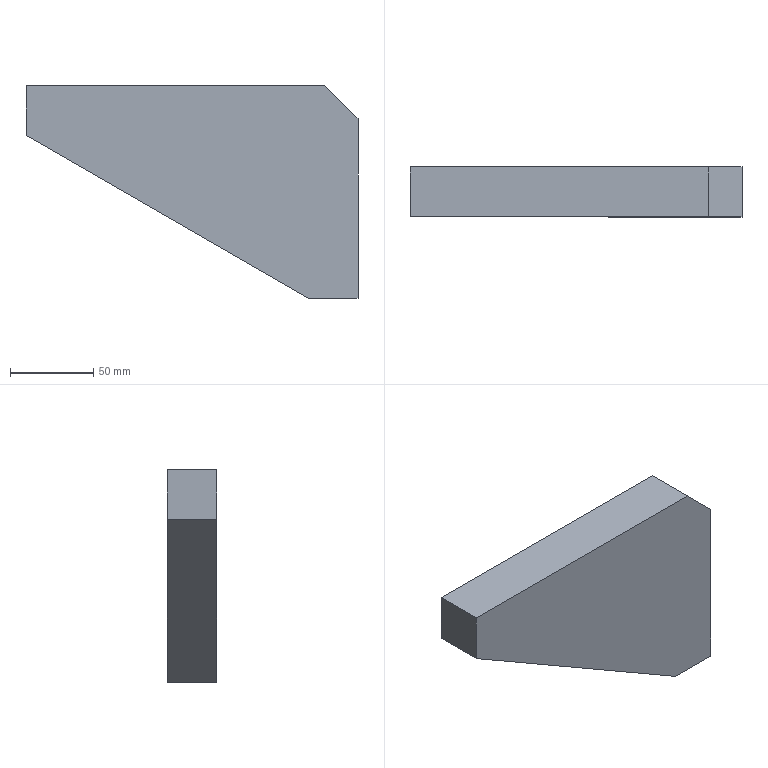Part | SolidWorks | features Extrusion 1 | 1 solid | 8 faces | box 200 x 30 x 128.15 mm | volume 512616 mm3 | plane 8
STEP:
#1=CARTESIAN_POINT('',(0.,0.,108.15));
#2=VERTEX_POINT('',#1);
#3=CARTESIAN_POINT('',(0.,0.,0.));
#4=VERTEX_POINT('',#3);
#5=CARTESIAN_POINT('',(0.,0.,108.15));
#6=DIRECTION('',(0.,0.,-1.));
#7=VECTOR('',#6,1000.);
#8=LINE('',#5,#7);
#9=EDGE_CURVE('',#2,#4,#8,.T.);
#10=ORIENTED_EDGE('',*,*,#9,.T.);
#11=CARTESIAN_POINT('',(0.,30.,0.));
#12=VERTEX_POINT('',#11);
#13=CARTESIAN_POINT('',(0.,30.,0.));
#14=DIRECTION('',(0.,-1.,0.));
#15=VECTOR('',#14,1000.);
#16=LINE('',#13,#15);
#17=EDGE_CURVE('',#12,#4,#16,.T.);
#18=ORIENTED_EDGE('',*,*,#17,.F.);
#19=CARTESIAN_POINT('',(0.,30.,108.15));
#20=VERTEX_POINT('',#19);
#21=CARTESIAN_POINT('',(0.,30.,108.15));
#22=DIRECTION('',(0.,0.,-1.));
#23=VECTOR('',#22,1000.);
#24=LINE('',#21,#23);
#25=EDGE_CURVE('',#20,#12,#24,.T.);
#26=ORIENTED_EDGE('',*,*,#25,.F.);
#27=CARTESIAN_POINT('',(0.,30.,108.15));
#28=DIRECTION('',(0.,-1.,0.));
#29=VECTOR('',#28,1000.);
#30=LINE('',#27,#29);
#31=EDGE_CURVE('',#20,#2,#30,.T.);
#32=ORIENTED_EDGE('',*,*,#31,.T.);
#33=EDGE_LOOP('',(#10,#18,#26,#32));
#34=FACE_OUTER_BOUND('',#33,.T.);
#35=CARTESIAN_POINT('',(0.,30.,108.15));
#36=DIRECTION('',(-1.,0.,0.));
#37=DIRECTION('',(0.,0.,1.));
#38=AXIS2_PLACEMENT_3D('',#35,#36,#37);
#39=PLANE('',#38);
#40=ADVANCED_FACE('',(#34),#39,.F.);
#41=CARTESIAN_POINT('',(-30.,0.,0.));
#42=VERTEX_POINT('',#41);
#43=CARTESIAN_POINT('',(0.,0.,0.));
#44=DIRECTION('',(-1.,0.,0.));
#45=VECTOR('',#44,1000.);
#46=LINE('',#43,#45);
#47=EDGE_CURVE('',#4,#42,#46,.T.);
#48=ORIENTED_EDGE('',*,*,#47,.T.);
#49=CARTESIAN_POINT('',(-30.,30.,0.));
#50=VERTEX_POINT('',#49);
#51=CARTESIAN_POINT('',(-30.,30.,0.));
#52=DIRECTION('',(0.,-1.,0.));
#53=VECTOR('',#52,1000.);
#54=LINE('',#51,#53);
#55=EDGE_CURVE('',#50,#42,#54,.T.);
#56=ORIENTED_EDGE('',*,*,#55,.F.);
#57=CARTESIAN_POINT('',(0.,30.,0.));
#58=DIRECTION('',(-1.,0.,0.));
#59=VECTOR('',#58,1000.);
#60=LINE('',#57,#59);
#61=EDGE_CURVE('',#12,#50,#60,.T.);
#62=ORIENTED_EDGE('',*,*,#61,.F.);
#63=ORIENTED_EDGE('',*,*,#17,.T.);
#64=EDGE_LOOP('',(#48,#56,#62,#63));
#65=FACE_OUTER_BOUND('',#64,.T.);
#66=CARTESIAN_POINT('',(0.,30.,0.));
#67=DIRECTION('',(0.,0.,1.));
#68=DIRECTION('',(1.,0.,0.));
#69=AXIS2_PLACEMENT_3D('',#66,#67,#68);
#70=PLANE('',#69);
#71=ADVANCED_FACE('',(#65),#70,.F.);
#72=CARTESIAN_POINT('',(-200.,0.,98.15));
#73=VERTEX_POINT('',#72);
#74=CARTESIAN_POINT('',(-30.,0.,0.));
#75=DIRECTION('',(-0.866,0.,0.5));
#76=VECTOR('',#75,1000.);
#77=LINE('',#74,#76);
#78=EDGE_CURVE('',#42,#73,#77,.T.);
#79=ORIENTED_EDGE('',*,*,#78,.T.);
#80=CARTESIAN_POINT('',(-200.,30.,98.15));
#81=VERTEX_POINT('',#80);
#82=CARTESIAN_POINT('',(-200.,30.,98.15));
#83=DIRECTION('',(0.,-1.,0.));
#84=VECTOR('',#83,1000.);
#85=LINE('',#82,#84);
#86=EDGE_CURVE('',#81,#73,#85,.T.);
#87=ORIENTED_EDGE('',*,*,#86,.F.);
#88=CARTESIAN_POINT('',(-30.,30.,0.));
#89=DIRECTION('',(-0.866,0.,0.5));
#90=VECTOR('',#89,1000.);
#91=LINE('',#88,#90);
#92=EDGE_CURVE('',#50,#81,#91,.T.);
#93=ORIENTED_EDGE('',*,*,#92,.F.);
#94=ORIENTED_EDGE('',*,*,#55,.T.);
#95=EDGE_LOOP('',(#79,#87,#93,#94));
#96=FACE_OUTER_BOUND('',#95,.T.);
#97=CARTESIAN_POINT('',(-30.,30.,0.));
#98=DIRECTION('',(0.5,0.,0.866));
#99=DIRECTION('',(0.866,0.,-0.5));
#100=AXIS2_PLACEMENT_3D('',#97,#98,#99);
#101=PLANE('',#100);
#102=ADVANCED_FACE('',(#96),#101,.F.);
#103=CARTESIAN_POINT('',(-200.,0.,128.15));
#104=VERTEX_POINT('',#103);
#105=CARTESIAN_POINT('',(-200.,0.,98.15));
#106=DIRECTION('',(0.,0.,1.));
#107=VECTOR('',#106,1000.);
#108=LINE('',#105,#107);
#109=EDGE_CURVE('',#73,#104,#108,.T.);
#110=ORIENTED_EDGE('',*,*,#109,.T.);
#111=CARTESIAN_POINT('',(-200.,30.,128.15));
#112=VERTEX_POINT('',#111);
#113=CARTESIAN_POINT('',(-200.,30.,128.15));
#114=DIRECTION('',(0.,-1.,0.));
#115=VECTOR('',#114,1000.);
#116=LINE('',#113,#115);
#117=EDGE_CURVE('',#112,#104,#116,.T.);
#118=ORIENTED_EDGE('',*,*,#117,.F.);
#119=CARTESIAN_POINT('',(-200.,30.,98.15));
#120=DIRECTION('',(0.,0.,1.));
#121=VECTOR('',#120,1000.);
#122=LINE('',#119,#121);
#123=EDGE_CURVE('',#81,#112,#122,.T.);
#124=ORIENTED_EDGE('',*,*,#123,.F.);
#125=ORIENTED_EDGE('',*,*,#86,.T.);
#126=EDGE_LOOP('',(#110,#118,#124,#125));
#127=FACE_OUTER_BOUND('',#126,.T.);
#128=CARTESIAN_POINT('',(-200.,30.,98.15));
#129=DIRECTION('',(1.,0.,0.));
#130=DIRECTION('',(0.,0.,-1.));
#131=AXIS2_PLACEMENT_3D('',#128,#129,#130);
#132=PLANE('',#131);
#133=ADVANCED_FACE('',(#127),#132,.F.);
#134=CARTESIAN_POINT('',(-20.,0.,128.15));
#135=VERTEX_POINT('',#134);
#136=CARTESIAN_POINT('',(-200.,0.,128.15));
#137=DIRECTION('',(1.,0.,0.));
#138=VECTOR('',#137,1000.);
#139=LINE('',#136,#138);
#140=EDGE_CURVE('',#104,#135,#139,.T.);
#141=ORIENTED_EDGE('',*,*,#140,.T.);
#142=CARTESIAN_POINT('',(-20.,30.,128.15));
#143=VERTEX_POINT('',#142);
#144=CARTESIAN_POINT('',(-20.,30.,128.15));
#145=DIRECTION('',(0.,-1.,0.));
#146=VECTOR('',#145,1000.);
#147=LINE('',#144,#146);
#148=EDGE_CURVE('',#143,#135,#147,.T.);
#149=ORIENTED_EDGE('',*,*,#148,.F.);
#150=CARTESIAN_POINT('',(-200.,30.,128.15));
#151=DIRECTION('',(1.,0.,0.));
#152=VECTOR('',#151,1000.);
#153=LINE('',#150,#152);
#154=EDGE_CURVE('',#112,#143,#153,.T.);
#155=ORIENTED_EDGE('',*,*,#154,.F.);
#156=ORIENTED_EDGE('',*,*,#117,.T.);
#157=EDGE_LOOP('',(#141,#149,#155,#156));
#158=FACE_OUTER_BOUND('',#157,.T.);
#159=CARTESIAN_POINT('',(-200.,30.,128.15));
#160=DIRECTION('',(0.,0.,-1.));
#161=DIRECTION('',(-1.,0.,0.));
#162=AXIS2_PLACEMENT_3D('',#159,#160,#161);
#163=PLANE('',#162);
#164=ADVANCED_FACE('',(#158),#163,.F.);
#165=CARTESIAN_POINT('',(-20.,0.,128.15));
#166=DIRECTION('',(0.7071,0.,-0.7071));
#167=VECTOR('',#166,1000.);
#168=LINE('',#165,#167);
#169=EDGE_CURVE('',#135,#2,#168,.T.);
#170=ORIENTED_EDGE('',*,*,#169,.T.);
#171=ORIENTED_EDGE('',*,*,#31,.F.);
#172=CARTESIAN_POINT('',(-20.,30.,128.15));
#173=DIRECTION('',(0.7071,0.,-0.7071));
#174=VECTOR('',#173,1000.);
#175=LINE('',#172,#174);
#176=EDGE_CURVE('',#143,#20,#175,.T.);
#177=ORIENTED_EDGE('',*,*,#176,.F.);
#178=ORIENTED_EDGE('',*,*,#148,.T.);
#179=EDGE_LOOP('',(#170,#171,#177,#178));
#180=FACE_OUTER_BOUND('',#179,.T.);
#181=CARTESIAN_POINT('',(-20.,30.,128.15));
#182=DIRECTION('',(-0.7071,0.,-0.7071));
#183=DIRECTION('',(-0.7071,0.,0.7071));
#184=AXIS2_PLACEMENT_3D('',#181,#182,#183);
#185=PLANE('',#184);
#186=ADVANCED_FACE('',(#180),#185,.F.);
#187=ORIENTED_EDGE('',*,*,#25,.T.);
#188=ORIENTED_EDGE('',*,*,#61,.T.);
#189=ORIENTED_EDGE('',*,*,#92,.T.);
#190=ORIENTED_EDGE('',*,*,#123,.T.);
#191=ORIENTED_EDGE('',*,*,#154,.T.);
#192=ORIENTED_EDGE('',*,*,#176,.T.);
#193=EDGE_LOOP('',(#187,#188,#189,#190,#191,#192));
#194=FACE_OUTER_BOUND('',#193,.T.);
#195=CARTESIAN_POINT('',(0.,30.,0.));
#196=DIRECTION('',(0.,1.,0.));
#197=DIRECTION('',(0.,0.,1.));
#198=AXIS2_PLACEMENT_3D('',#195,#196,#197);
#199=PLANE('',#198);
#200=ADVANCED_FACE('',(#194),#199,.T.);
#201=ORIENTED_EDGE('',*,*,#9,.F.);
#202=ORIENTED_EDGE('',*,*,#169,.F.);
#203=ORIENTED_EDGE('',*,*,#140,.F.);
#204=ORIENTED_EDGE('',*,*,#109,.F.);
#205=ORIENTED_EDGE('',*,*,#78,.F.);
#206=ORIENTED_EDGE('',*,*,#47,.F.);
#207=EDGE_LOOP('',(#201,#202,#203,#204,#205,#206));
#208=FACE_OUTER_BOUND('',#207,.T.);
#209=CARTESIAN_POINT('',(0.,0.,0.));
#210=DIRECTION('',(0.,1.,0.));
#211=DIRECTION('',(0.,0.,1.));
#212=AXIS2_PLACEMENT_3D('',#209,#210,#211);
#213=PLANE('',#212);
#214=ADVANCED_FACE('',(#208),#213,.F.);
#215=CLOSED_SHELL('',(#40,#71,#102,#133,#164,#186,#200,#214));
#216=MANIFOLD_SOLID_BREP('',#215);
#217=CARTESIAN_POINT('',(0.,0.,0.));
#218=DIRECTION('',(0.,0.,1.));
#219=DIRECTION('',(1.,0.,0.));
#220=AXIS2_PLACEMENT_3D('',#217,#218,#219);
#221=(LENGTH_UNIT()NAMED_UNIT(*)SI_UNIT(.MILLI.,.METRE.));
#222=UNCERTAINTY_MEASURE_WITH_UNIT(LENGTH_MEASURE(0.00001),#221,'','');
#223=(NAMED_UNIT(*)PLANE_ANGLE_UNIT()SI_UNIT($,.RADIAN.));
#224=(NAMED_UNIT(*)SI_UNIT($,.STERADIAN.)SOLID_ANGLE_UNIT());
#225=(GEOMETRIC_REPRESENTATION_CONTEXT(3)GLOBAL_UNCERTAINTY_ASSIGNED_CONTEXT((#222))GLOBAL_UNIT_ASSIGNED_CONTEXT((#221,#223,#224))REPRESENTATION_CONTEXT('',''));
#226=ADVANCED_BREP_SHAPE_REPRESENTATION('',(#216,#220),#225);